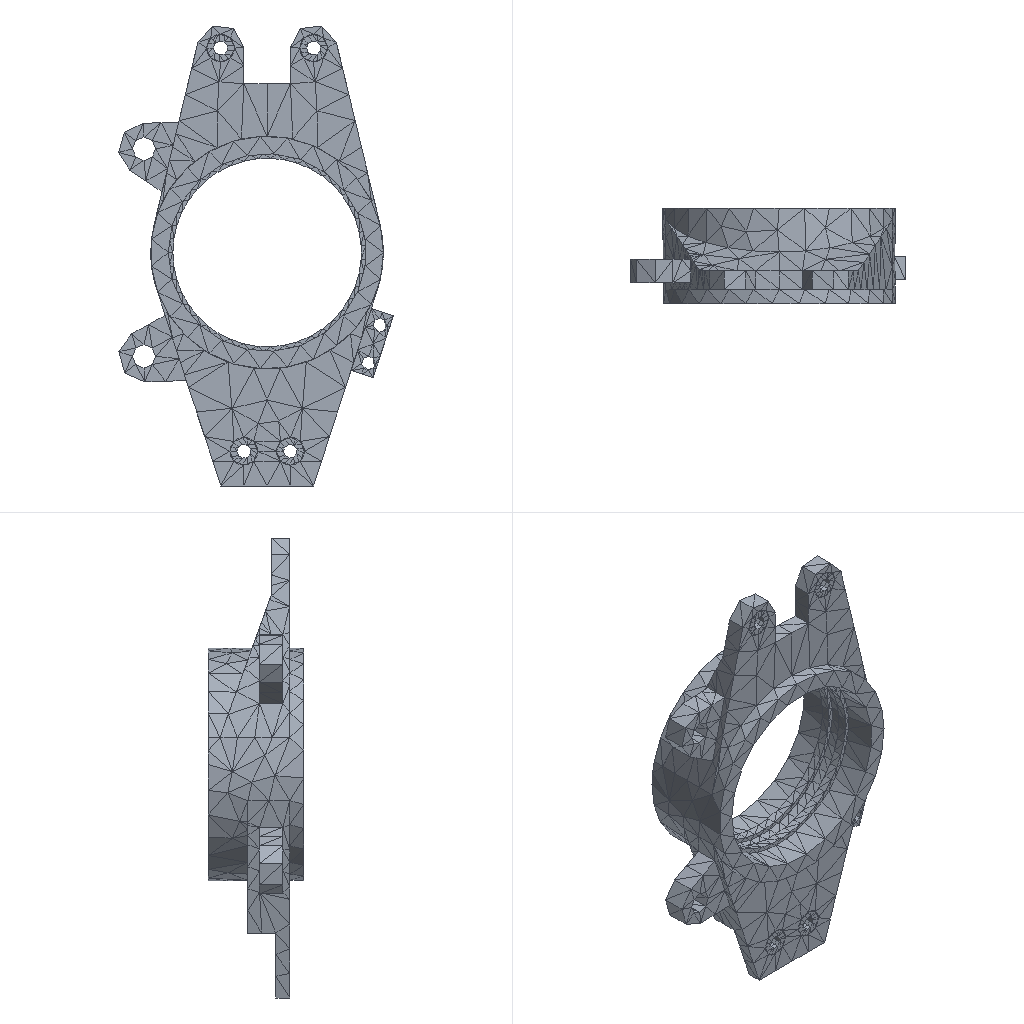Simulation study | ansys workbench
Ansys APDL input file, long lists of numbers shortened:
/batch
/config,noeldb,1     ! force off writing results to database
*get,_wallstrt,active,,time,wall
! ANSYS input file written by Workbench version 2022 R1
! File used for geometry attach:
/title,__1--____ (C5)
! ****** Begin Custom Load Command Snippet ******
/COM, ACT Extensions:
/COM,     LSDYNA, 2021.1
/COM,
! ****** End   Custom Load Command Snippet ******
*DIM,_wb_ProjectScratch_dir,string,248
_wb_ProjectScratch_dir(1) = ''
*DIM,_wb_SolverFiles_dir,string,248
_wb_SolverFiles_dir(1) = ''
*DIM,_wb_userfiles_dir,string,248
_wb_userfiles_dir(1) = ''
/com,--- Data in consistent NMM units. See Solving Units in the help system for more information.
/units,MPA
/nopr
/wb,file,start              !  signify a WB generated input file
/prep7
! Turn off shape checking because checks already performed inside WB mesher.
! See help system for more information.
SHPP,OFF,,NOWARN
/nolist
etcon,set             ! allow ANSYS to choose best KEYOP's for 180x elements, resets any applicable keyopt to MAPDL defaults
/com,*********** Nodes for the whole assembly ***********
nblock,3,,8127
(1i9,3e20.9e3)
        1    -1.253072820E+01    -1.049943652E+01    -8.837560534E+01
! (7388 more lines like these left out)
-1
/com,*********** Nodes for all Remote Points ***********
nblock,3
(1i9,3e20.9e3)
     7390     4.187219516E-04     9.308146968E+00     5.345567280E+00
-1
/wb,elem,start            !  set before creation of elements
/com,*********** Elements for Body 1 "SYS\fix_end 2" ***********
et,1,186
keyo,1,2,1          ! set full integration on SOLID186
eblock,19,solid,,76
(19i9)
        1        1        1        1        0        0        0        0       20        0       58      391      495      494      426      394      529      510      450
! (151 more lines like these left out)
-1
/com,*********** Elements for Body 2 "SYS\fix_end 3" ***********
et,2,186
keyo,2,2,1          ! set full integration on SOLID186
eblock,19,solid,,76
(19i9)
        2        2        2        2        0        0        0        0       20        0      191     1324     1348     1349     1325     1336     1404     1403     1337
! (151 more lines like these left out)
-1
/com,*********** Elements for Body 3 "SYS\fix_end 4" ***********
et,3,186
keyo,3,2,1          ! set full integration on SOLID186
eblock,19,solid,,57
(19i9)
        3        3        3        3        0        0        0        0       20        0        1       45       68       69       46       60      103      104       59
! (113 more lines like these left out)
-1
/com,*********** Elements for Body 4 "SYS\fix_end 1" ***********
et,4,186
keyo,4,2,1          ! set full integration on SOLID186
eblock,19,solid,,57
(19i9)
        4        4        4        4        0        0        0        0       20        0      134      930      953      954      931      945      988      989      944
! (113 more lines like these left out)
-1
/com,*********** Elements for Body 5 "SYS\qianzhuan" ***********
et,5,187
eblock,19,solid,,2770
(19i9)
        5        5        5        5        0        0        0        0       10        0      267     1940     1947     1957     2732     3818     3885     3819     3821
! (5539 more lines like these left out)
-1
/wb,elem,end               !  done creating elements
/com,*********** Send User Defined Coordinate System(s) ***********
csys,0
toffst,273.15,  ! Temperature offset from absolute zero
/com,*********** Set Reference Temperature ***********
tref,22.
/wb,mat,start              !  starting to send materials
/com,*********** Send Materials ***********
MP,EX,1,68950,	! tonne s^-2 mm^-1
MP,NUXY,1,0.33,
MP,DENS,1,2.7e-09,	! tonne mm^-3
MP,ALPX,1,7.88860905221012e-31,	! C^-1
! (31 more lines like these left out)
/wb,mat,end                !  done sending materials
!************************* Model Summary ********************
!SYS\fix_end 2,	Aluminum 6061-T6; 6061-T651,	matid,	1
!SYS\fix_end 3,	Aluminum 6061-T6; 6061-T651,	matid,	2
!SYS\fix_end 4,	Aluminum 6061-T6; 6061-T651,	matid,	3
!SYS\fix_end 1,	Aluminum 6061-T6; 6061-T651,	matid,	4
!SYS\qianzhuan,	Aluminum 6061-T6; 6061-T651,	matid,	5
!************************* End Model Summary ********************
! get the diagonal of the bounding box. Needed later for other things
*get,_xmin,node,,mnloc,x
*get,_ymin,node,,mnloc,y
*get,_zmin,node,,mnloc,z
*get,_xmax,node,,mxloc,x
*get,_ymax,node,,mxloc,y
*get,_zmax,node,,mxloc,z
_ASMDIAG=(_xmax-_xmin)*(_xmax-_xmin)+(_ymax-_ymin)*(_ymax-_ymin)+(_zmax-_zmin)*(_zmax-_zmin)
_ASMDIAG=SQRT(_ASMDIAG)
/wb,contact,start          !  starting to send contact
/com,*********** Create Contact "接触区域" ***********
/com,            Real Constant Set For Above Contact Is 7 & 6
*set,tid,7
*set,cid,6
r,tid
r,cid
et,tid,170
et,cid,174
eblock,10,,,68
(15i9)
     5356        7        7        7        0      415      400      511      462      578      580      769      624
! (67 more lines like these left out)
-1
eblock,10,,,68
(15i9)
     5424        6        6        6        0      415      400      511      462      578      580      769      624
! (67 more lines like these left out)
-1
eblock,10,,,16
(15i9)
     5492        6        7        6        0     1806     1809     1820     1820     2991     3013     1820     2995
! (15 more lines like these left out)
-1
eblock,10,,,16
(15i9)
     5508        7        6        7        0     1806     1809     1820     1820     2991     3013     1820     2995
! (15 more lines like these left out)
-1
keyo,cid,8,2               ! auto create asymmetric contact (from Program Controlled setting)
keyo,cid,10,0              ! adjust contact stiffness each NR iteration (from Program Controlled setting)
keyo,cid,12,5              ! bonded always
keyo,cid,18,1              ! small sliding turned on by application
keyo,cid,2,0               ! augmented Lagrange (from Program Controlled setting)
keyo,cid,4,0               ! on Gauss point (from Program Controlled setting)
keyo,cid,9,1               ! ignore initial gaps/penetration
keyo,cid,7,0               ! No Prediction
rmod,tid,3,10.      ! FKN
rmod,tid,5,0.       ! ICONT
rmod,tid,6,0.       ! PINB
rmod,tid,10,0.      ! CNOF
rmod,tid,12,0.      ! FKT
rmod,tid,36,39      ! WB DSID
rmod,cid,3,10.      ! FKN
rmod,cid,5,0.       ! ICONT
rmod,cid,6,0.       ! PINB
rmod,cid,10,0.      ! CNOF
rmod,cid,12,0.      ! FKT
rmod,cid,36,39      ! WB DSID
/com,*********** Create Contact "接触区域 2" ***********
/com,            Real Constant Set For Above Contact Is 9 & 8
*set,tid,9
*set,cid,8
r,tid
r,cid
et,tid,170
et,cid,174
eblock,10,,,68
(15i9)
     5524        9        9        9        0     1390     1391     1392     1342     1737     1739     1641     1640
! (67 more lines like these left out)
-1
eblock,10,,,68
(15i9)
     5592        8        8        8        0     1390     1391     1392     1342     1737     1739     1641     1640
! (67 more lines like these left out)
-1
eblock,10,,,16
(15i9)
     5660        8        9        8        0     1790     1793     1800     1800     2910     2930     1800     2912
! (15 more lines like these left out)
-1
eblock,10,,,16
(15i9)
     5676        9        8        9        0     1790     1793     1800     1800     2910     2930     1800     2912
! (15 more lines like these left out)
-1
keyo,cid,8,2               ! auto create asymmetric contact (from Program Controlled setting)
keyo,cid,10,0              ! adjust contact stiffness each NR iteration (from Program Controlled setting)
keyo,cid,12,5              ! bonded always
keyo,cid,18,1              ! small sliding turned on by application
keyo,cid,2,0               ! augmented Lagrange (from Program Controlled setting)
keyo,cid,4,0               ! on Gauss point (from Program Controlled setting)
keyo,cid,9,1               ! ignore initial gaps/penetration
keyo,cid,7,0               ! No Prediction
rmod,tid,3,10.      ! FKN
rmod,tid,5,0.       ! ICONT
rmod,tid,6,0.       ! PINB
rmod,tid,10,0.      ! CNOF
rmod,tid,12,0.      ! FKT
rmod,tid,36,42      ! WB DSID
rmod,cid,3,10.      ! FKN
rmod,cid,5,0.       ! ICONT
rmod,cid,6,0.       ! PINB
rmod,cid,10,0.      ! CNOF
rmod,cid,12,0.      ! FKT
rmod,cid,36,42      ! WB DSID
/com,*********** Create Contact "接触区域 3" ***********
/com,            Real Constant Set For Above Contact Is 11 & 10
*set,tid,11
*set,cid,10
r,tid
r,cid
et,tid,170
et,cid,174
eblock,10,,,51
(15i9)
     5692       11       11       11        0       94       95       96       62      366      368      303      302
! (50 more lines like these left out)
-1
eblock,10,,,51
(15i9)
     5743       10       10       10        0       94       95       96       62      366      368      303      302
! (50 more lines like these left out)
-1
eblock,10,,,16
(15i9)
     5794       10       11       10        0     1779     1775     1786     1786     2839     2841     1786     2861
! (15 more lines like these left out)
-1
eblock,10,,,16
(15i9)
     5810       11       10       11        0     1779     1775     1786     1786     2839     2841     1786     2861
! (15 more lines like these left out)
-1
keyo,cid,8,2               ! auto create asymmetric contact (from Program Controlled setting)
keyo,cid,10,0              ! adjust contact stiffness each NR iteration (from Program Controlled setting)
keyo,cid,12,5              ! bonded always
keyo,cid,18,1              ! small sliding turned on by application
keyo,cid,2,0               ! augmented Lagrange (from Program Controlled setting)
keyo,cid,4,0               ! on Gauss point (from Program Controlled setting)
keyo,cid,9,1               ! ignore initial gaps/penetration
keyo,cid,7,0               ! No Prediction
rmod,tid,3,10.      ! FKN
rmod,tid,5,0.       ! ICONT
rmod,tid,6,0.       ! PINB
rmod,tid,10,0.      ! CNOF
rmod,tid,12,0.      ! FKT
rmod,tid,36,45      ! WB DSID
rmod,cid,3,10.      ! FKN
rmod,cid,5,0.       ! ICONT
rmod,cid,6,0.       ! PINB
rmod,cid,10,0.      ! CNOF
rmod,cid,12,0.      ! FKT
rmod,cid,36,45      ! WB DSID
/com,*********** Create Contact "接触区域 4" ***********
/com,            Real Constant Set For Above Contact Is 13 & 12
*set,tid,13
*set,cid,12
r,tid
r,cid
et,tid,170
et,cid,174
eblock,10,,,51
(15i9)
     5826       13       13       13        0      979      980      981      947     1251     1253     1188     1187
! (50 more lines like these left out)
-1
eblock,10,,,51
(15i9)
     5877       12       12       12        0      979      980      981      947     1251     1253     1188     1187
! (50 more lines like these left out)
-1
eblock,10,,,16
(15i9)
     5928       12       13       12        0     1761     1765     1772     1772     2763     2793     1772     2765
! (15 more lines like these left out)
-1
eblock,10,,,16
(15i9)
     5944       13       12       13        0     1761     1765     1772     1772     2763     2793     1772     2765
! (15 more lines like these left out)
-1
keyo,cid,8,2               ! auto create asymmetric contact (from Program Controlled setting)
keyo,cid,10,0              ! adjust contact stiffness each NR iteration (from Program Controlled setting)
keyo,cid,12,5              ! bonded always
keyo,cid,18,1              ! small sliding turned on by application
keyo,cid,2,0               ! augmented Lagrange (from Program Controlled setting)
keyo,cid,4,0               ! on Gauss point (from Program Controlled setting)
keyo,cid,9,1               ! ignore initial gaps/penetration
keyo,cid,7,0               ! No Prediction
rmod,tid,3,10.      ! FKN
rmod,tid,5,0.       ! ICONT
rmod,tid,6,0.       ! PINB
rmod,tid,10,0.      ! CNOF
rmod,tid,12,0.      ! FKT
rmod,tid,36,48      ! WB DSID
rmod,cid,3,10.      ! FKN
rmod,cid,5,0.       ! ICONT
rmod,cid,6,0.       ! PINB
rmod,cid,10,0.      ! CNOF
rmod,cid,12,0.      ! FKT
rmod,cid,36,48      ! WB DSID
nsel,all
esel,all
/wb,contact,end            !  done creating contacts
/golist
/wb,load,start             !  starting to send loads
/com,*********** Fixed Supports ***********
CMBLOCK,_FIXEDSU,NODE,      498
(8i10)
        26        27        28        29        30        31        32        33
! (62 more lines like these left out)
cmsel,s,_FIXEDSU
d,all,all
nsel,all
/com,*********** Create Remote Point "内部远程点" ***********
! -------- Remote Point Used by "力矩" --------
*set,tid,15
*set,cid,14
et,cid,177
et,tid,170
keyo,tid,2,1               ! Don't fix the pilot node
keyo,tid,4,111111
keyo,cid,12,5              ! Bonded Contact
keyo,cid,4,1               ! Deformable RBE3 style load
keyo,cid,2,2               ! MPC style contact
eblock,10,,,121
(15i9)
     5960       14       14       14        0     2063     2076     4738
! (120 more lines like these left out)
-1
*set,_npilot,7390
_npilot57=_npilot
type,tid
mat ,cid
real,cid
tshape,pilo
en,6081,_npilot
tshape
/com,*********** Construct Moment Using Remote Attachment ***********
/gst,on,on
fini
*get,_numnode,node,0,count
*get,_numelem,elem,0,count
*get, _MAXELEMNUM, elem, 0, NUM, MAX
*get, _MAXNODENUM, node, 0, NUM, MAX
*get, _MAXELEMTYPE, etyp, 0, NUM, MAX
*get, _MAXREALCONST, real, 0, NUM, MAX
/go
/wb,load,end               !  done creating loads
/com,--- Number of total nodes = %_numnode%
/com,--- Number of contact elements = 725
/com,--- Number of spring elements = 0
/com,--- Number of bearing elements = 0
/com,--- Number of solid elements = 3036
/com,--- Number of condensed parts = 0
/com,--- Number of total elements = %_numelem%
*get,_wallbsol,active,,time,wall
/com,****************************************************************************
/com,*************************    SOLUTION       ********************************
/com,****************************************************************************
/solu
antype,0                   ! static analysis
_thickRatio=0.2     ! Ratio of thick parts in the model
eqsl,sparse,,,,,1
cntr,print,1               ! print out contact info and also make no initial contact an error
dmpoption,emat,no             ! Don't combine emat file for DANSYS
dmpoption,esav,no             ! Don't combine esav file for DANSYS
nldiag,cont,iter           ! print out contact info each equilibrium iteration
rescontrol,,none                 ! Do not keep any restart files
/com,****************************************************
/com,******************* SOLVE FOR LS 1 OF 1 ****************
nsel,s,node,,7390
f,all,mx,0.
f,all,my,288.
f,all,mz,0.
nsel,all
/nopr
/gopr
nsub,1,1,1
time,1.
outres,erase
outres,all,none
outres,nsol,all,
outres,rsol,all
outres,eangl,all
outres,etmp,all
outres,veng,all
outres,strs,all,
outres,epel,all,
outres,eppl,all,
outres,cont,all,
! *********** WB SOLVE COMMAND ***********
! check interactive state
*get,ANSINTER_,active,,int
*if,ANSINTER_,ne,0,then
/eof
*endif
solve
/com *************** Write FE CONNECTORS *********
CEWRITE,file,ce,,INTE
/com,****************************************************
/com,*************** FINISHED SOLVE FOR LS 1 *************
*get,_wallasol,active,,time,wall
/nopr
*get,_numnode,node,0,count
*get,_numelem,elem,0,count
*get, _MAXELEMNUM, elem, 0, NUM, MAX
*get, _MAXNODENUM, node, 0, NUM, MAX,,,INTERNAL
*get, _MAXELEMTYPE, etyp, 0, NUM, MAX
*get, _MAXREALCONST, real, 0, NUM, MAX
/gopr
/post1
xmlo,ENCODING,ISO-8859-1
xmlo,parm
/xml,parm,xml
fini
/gopr
*get,_walldone,active,,time,wall
_preptime=(_wallbsol-_wallstrt)*3600
_solvtime=(_wallasol-_wallbsol)*3600
_posttime=(_walldone-_wallasol)*3600
_totaltim=(_walldone-_wallstrt)*3600
*get,_dlbratio,active,0,solu,dlbr
*get,_combtime,active,0,solu,comb
*get,_ssmode,active,0,solu,ssmm
*get,_ndofs,active,0,solu,ndof
*get,_sol_end_time,active,0,set,time
*if,_sol_end_time,eq,1.,then
/fclean				!clean distributed files
*endif
/com,--- Total number of nodes = %_numnode%
/com,--- Total number of elements = %_numelem%
/com,--- Element load balance ratio = %_dlbratio%
/com,--- Time to combine distributed files = %_combtime%
/com,--- Sparse memory mode = %_ssmode%
/com,--- Number of DOF = %_ndofs%
/wb,file,end               ! done with WB generated input